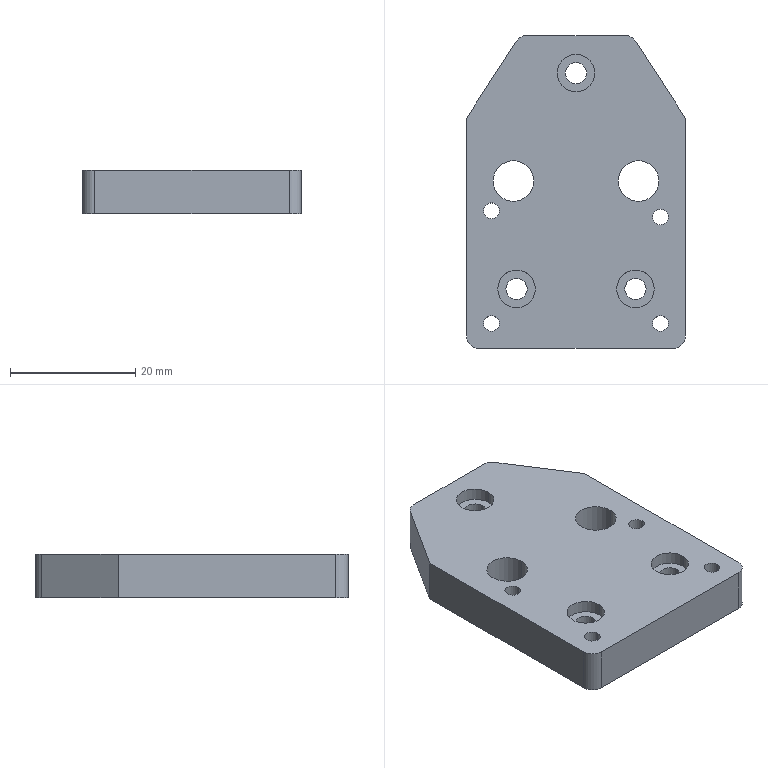Part | STEP file | 11-FG-SB00811 | 1 solid | 48 faces | box 35 x 50 x 7 mm | volume 10258 mm3 | cylinder 34 | plane 14 | commonest cylinder face diameters 2.5 x8 3.4 x6 6 x6 6.5 x6 4 x4 7 x4
STEP:
#1=CARTESIAN_POINT('',(13.25,14.24,7.));
#2=VERTEX_POINT('',#1);
#3=CARTESIAN_POINT('',(6.75,14.24,7.));
#4=VERTEX_POINT('',#3);
#5=CARTESIAN_POINT('',(10.,14.24,7.));
#6=DIRECTION('',(0.,0.,-1.));
#7=DIRECTION('',(-1.,0.,0.));
#8=AXIS2_PLACEMENT_3D('',#5,#6,#7);
#9=CIRCLE('',#8,3.25);
#10=EDGE_CURVE('',#2,#4,#9,.T.);
#11=ORIENTED_EDGE('',*,*,#10,.F.);
#12=CARTESIAN_POINT('',(13.25,14.24,0.));
#13=VERTEX_POINT('',#12);
#14=CARTESIAN_POINT('',(13.25,14.24,7.));
#15=DIRECTION('',(0.,0.,-1.));
#16=VECTOR('',#15,1000.);
#17=LINE('',#14,#16);
#18=EDGE_CURVE('',#2,#13,#17,.T.);
#19=ORIENTED_EDGE('',*,*,#18,.T.);
#20=CARTESIAN_POINT('',(6.75,14.24,0.));
#21=VERTEX_POINT('',#20);
#22=CARTESIAN_POINT('',(10.,14.24,0.));
#23=DIRECTION('',(0.,0.,-1.));
#24=DIRECTION('',(-1.,0.,0.));
#25=AXIS2_PLACEMENT_3D('',#22,#23,#24);
#26=CIRCLE('',#25,3.25);
#27=EDGE_CURVE('',#13,#21,#26,.T.);
#28=ORIENTED_EDGE('',*,*,#27,.T.);
#29=CARTESIAN_POINT('',(6.75,14.24,7.));
#30=DIRECTION('',(0.,0.,-1.));
#31=VECTOR('',#30,1000.);
#32=LINE('',#29,#31);
#33=EDGE_CURVE('',#4,#21,#32,.T.);
#34=ORIENTED_EDGE('',*,*,#33,.F.);
#35=EDGE_LOOP('',(#11,#19,#28,#34));
#36=FACE_OUTER_BOUND('',#35,.T.);
#37=CARTESIAN_POINT('',(10.,14.24,7.));
#38=DIRECTION('',(0.,0.,-1.));
#39=DIRECTION('',(-1.,0.,0.));
#40=AXIS2_PLACEMENT_3D('',#37,#38,#39);
#41=CYLINDRICAL_SURFACE('',#40,3.25);
#42=ADVANCED_FACE('',(#36),#41,.F.);
#43=CARTESIAN_POINT('',(-6.75,14.24,7.));
#44=VERTEX_POINT('',#43);
#45=CARTESIAN_POINT('',(-13.25,14.24,7.));
#46=VERTEX_POINT('',#45);
#47=CARTESIAN_POINT('',(-10.,14.24,7.));
#48=DIRECTION('',(0.,0.,-1.));
#49=DIRECTION('',(-1.,0.,0.));
#50=AXIS2_PLACEMENT_3D('',#47,#48,#49);
#51=CIRCLE('',#50,3.25);
#52=EDGE_CURVE('',#44,#46,#51,.T.);
#53=ORIENTED_EDGE('',*,*,#52,.F.);
#54=CARTESIAN_POINT('',(-6.75,14.24,0.));
#55=VERTEX_POINT('',#54);
#56=CARTESIAN_POINT('',(-6.75,14.24,7.));
#57=DIRECTION('',(0.,0.,-1.));
#58=VECTOR('',#57,1000.);
#59=LINE('',#56,#58);
#60=EDGE_CURVE('',#44,#55,#59,.T.);
#61=ORIENTED_EDGE('',*,*,#60,.T.);
#62=CARTESIAN_POINT('',(-13.25,14.24,0.));
#63=VERTEX_POINT('',#62);
#64=CARTESIAN_POINT('',(-10.,14.24,0.));
#65=DIRECTION('',(0.,0.,-1.));
#66=DIRECTION('',(-1.,0.,0.));
#67=AXIS2_PLACEMENT_3D('',#64,#65,#66);
#68=CIRCLE('',#67,3.25);
#69=EDGE_CURVE('',#55,#63,#68,.T.);
#70=ORIENTED_EDGE('',*,*,#69,.T.);
#71=CARTESIAN_POINT('',(-13.25,14.24,7.));
#72=DIRECTION('',(0.,0.,-1.));
#73=VECTOR('',#72,1000.);
#74=LINE('',#71,#73);
#75=EDGE_CURVE('',#46,#63,#74,.T.);
#76=ORIENTED_EDGE('',*,*,#75,.F.);
#77=EDGE_LOOP('',(#53,#61,#70,#76));
#78=FACE_OUTER_BOUND('',#77,.T.);
#79=CARTESIAN_POINT('',(-10.,14.24,7.));
#80=DIRECTION('',(0.,0.,-1.));
#81=DIRECTION('',(-1.,0.,0.));
#82=AXIS2_PLACEMENT_3D('',#79,#80,#81);
#83=CYLINDRICAL_SURFACE('',#82,3.25);
#84=ADVANCED_FACE('',(#78),#83,.F.);
#85=CARTESIAN_POINT('',(3.25,31.5,3.4));
#86=VERTEX_POINT('',#85);
#87=CARTESIAN_POINT('',(-3.25,31.5,3.4));
#88=VERTEX_POINT('',#87);
#89=CARTESIAN_POINT('',(0.,31.5,3.4));
#90=DIRECTION('',(0.,0.,-1.));
#91=DIRECTION('',(-1.,0.,0.));
#92=AXIS2_PLACEMENT_3D('',#89,#90,#91);
#93=CIRCLE('',#92,3.25);
#94=EDGE_CURVE('',#86,#88,#93,.T.);
#95=ORIENTED_EDGE('',*,*,#94,.F.);
#96=CARTESIAN_POINT('',(3.25,31.5,0.));
#97=VERTEX_POINT('',#96);
#98=CARTESIAN_POINT('',(3.25,31.5,0.));
#99=DIRECTION('',(0.,0.,-1.));
#100=VECTOR('',#99,1000.);
#101=LINE('',#98,#100);
#102=EDGE_CURVE('',#86,#97,#101,.T.);
#103=ORIENTED_EDGE('',*,*,#102,.T.);
#104=CARTESIAN_POINT('',(-3.25,31.5,0.));
#105=VERTEX_POINT('',#104);
#106=CARTESIAN_POINT('',(0.,31.5,0.));
#107=DIRECTION('',(0.,0.,-1.));
#108=DIRECTION('',(-1.,0.,0.));
#109=AXIS2_PLACEMENT_3D('',#106,#107,#108);
#110=CIRCLE('',#109,3.25);
#111=EDGE_CURVE('',#97,#105,#110,.T.);
#112=ORIENTED_EDGE('',*,*,#111,.T.);
#113=CARTESIAN_POINT('',(-3.25,31.5,0.));
#114=DIRECTION('',(0.,0.,-1.));
#115=VECTOR('',#114,1000.);
#116=LINE('',#113,#115);
#117=EDGE_CURVE('',#88,#105,#116,.T.);
#118=ORIENTED_EDGE('',*,*,#117,.F.);
#119=EDGE_LOOP('',(#95,#103,#112,#118));
#120=FACE_OUTER_BOUND('',#119,.T.);
#121=CARTESIAN_POINT('',(0.,31.5,0.));
#122=DIRECTION('',(0.,0.,-1.));
#123=DIRECTION('',(-1.,0.,0.));
#124=AXIS2_PLACEMENT_3D('',#121,#122,#123);
#125=CYLINDRICAL_SURFACE('',#124,3.25);
#126=ADVANCED_FACE('',(#120),#125,.F.);
#127=CARTESIAN_POINT('',(-1.7,31.5,5.));
#128=VERTEX_POINT('',#127);
#129=CARTESIAN_POINT('',(1.7,31.5,5.));
#130=VERTEX_POINT('',#129);
#131=CARTESIAN_POINT('',(0.,31.5,5.));
#132=DIRECTION('',(0.,0.,1.));
#133=DIRECTION('',(1.,0.,0.));
#134=AXIS2_PLACEMENT_3D('',#131,#132,#133);
#135=CIRCLE('',#134,1.7);
#136=EDGE_CURVE('',#128,#130,#135,.T.);
#137=ORIENTED_EDGE('',*,*,#136,.T.);
#138=CARTESIAN_POINT('',(1.7,31.5,3.4));
#139=VERTEX_POINT('',#138);
#140=CARTESIAN_POINT('',(1.7,31.5,0.));
#141=DIRECTION('',(0.,0.,-1.));
#142=VECTOR('',#141,1000.);
#143=LINE('',#140,#142);
#144=EDGE_CURVE('',#130,#139,#143,.T.);
#145=ORIENTED_EDGE('',*,*,#144,.T.);
#146=CARTESIAN_POINT('',(-1.7,31.5,3.4));
#147=VERTEX_POINT('',#146);
#148=CARTESIAN_POINT('',(0.,31.5,3.4));
#149=DIRECTION('',(0.,0.,-1.));
#150=DIRECTION('',(-1.,0.,0.));
#151=AXIS2_PLACEMENT_3D('',#148,#149,#150);
#152=CIRCLE('',#151,1.7);
#153=EDGE_CURVE('',#139,#147,#152,.T.);
#154=ORIENTED_EDGE('',*,*,#153,.T.);
#155=CARTESIAN_POINT('',(-1.7,31.5,0.));
#156=DIRECTION('',(0.,0.,-1.));
#157=VECTOR('',#156,1000.);
#158=LINE('',#155,#157);
#159=EDGE_CURVE('',#128,#147,#158,.T.);
#160=ORIENTED_EDGE('',*,*,#159,.F.);
#161=EDGE_LOOP('',(#137,#145,#154,#160));
#162=FACE_OUTER_BOUND('',#161,.T.);
#163=CARTESIAN_POINT('',(0.,31.5,0.));
#164=DIRECTION('',(0.,0.,-1.));
#165=DIRECTION('',(-1.,0.,0.));
#166=AXIS2_PLACEMENT_3D('',#163,#164,#165);
#167=CYLINDRICAL_SURFACE('',#166,1.7);
#168=ADVANCED_FACE('',(#162),#167,.F.);
#169=CARTESIAN_POINT('',(-3.,31.5,5.));
#170=VERTEX_POINT('',#169);
#171=CARTESIAN_POINT('',(3.,31.5,5.));
#172=VERTEX_POINT('',#171);
#173=CARTESIAN_POINT('',(0.,31.5,5.));
#174=DIRECTION('',(0.,0.,1.));
#175=DIRECTION('',(1.,0.,0.));
#176=AXIS2_PLACEMENT_3D('',#173,#174,#175);
#177=CIRCLE('',#176,3.);
#178=EDGE_CURVE('',#170,#172,#177,.T.);
#179=ORIENTED_EDGE('',*,*,#178,.F.);
#180=CARTESIAN_POINT('',(-3.,31.5,7.));
#181=VERTEX_POINT('',#180);
#182=CARTESIAN_POINT('',(-3.,31.5,5.));
#183=DIRECTION('',(0.,0.,1.));
#184=VECTOR('',#183,1000.);
#185=LINE('',#182,#184);
#186=EDGE_CURVE('',#170,#181,#185,.T.);
#187=ORIENTED_EDGE('',*,*,#186,.T.);
#188=CARTESIAN_POINT('',(3.,31.5,7.));
#189=VERTEX_POINT('',#188);
#190=CARTESIAN_POINT('',(0.,31.5,7.));
#191=DIRECTION('',(0.,0.,1.));
#192=DIRECTION('',(1.,0.,0.));
#193=AXIS2_PLACEMENT_3D('',#190,#191,#192);
#194=CIRCLE('',#193,3.);
#195=EDGE_CURVE('',#181,#189,#194,.T.);
#196=ORIENTED_EDGE('',*,*,#195,.T.);
#197=CARTESIAN_POINT('',(3.,31.5,5.));
#198=DIRECTION('',(0.,0.,1.));
#199=VECTOR('',#198,1000.);
#200=LINE('',#197,#199);
#201=EDGE_CURVE('',#172,#189,#200,.T.);
#202=ORIENTED_EDGE('',*,*,#201,.F.);
#203=EDGE_LOOP('',(#179,#187,#196,#202));
#204=FACE_OUTER_BOUND('',#203,.T.);
#205=CARTESIAN_POINT('',(0.,31.5,5.));
#206=DIRECTION('',(0.,0.,1.));
#207=DIRECTION('',(1.,0.,0.));
#208=AXIS2_PLACEMENT_3D('',#205,#206,#207);
#209=CYLINDRICAL_SURFACE('',#208,3.);
#210=ADVANCED_FACE('',(#204),#209,.F.);
#211=CARTESIAN_POINT('',(-12.25,-8.5,7.));
#212=VERTEX_POINT('',#211);
#213=CARTESIAN_POINT('',(-14.75,-8.5,7.));
#214=VERTEX_POINT('',#213);
#215=CARTESIAN_POINT('',(-13.5,-8.5,7.));
#216=DIRECTION('',(0.,0.,-1.));
#217=DIRECTION('',(-1.,0.,0.));
#218=AXIS2_PLACEMENT_3D('',#215,#216,#217);
#219=CIRCLE('',#218,1.25);
#220=EDGE_CURVE('',#212,#214,#219,.T.);
#221=ORIENTED_EDGE('',*,*,#220,.F.);
#222=CARTESIAN_POINT('',(-12.25,-8.5,0.));
#223=VERTEX_POINT('',#222);
#224=CARTESIAN_POINT('',(-12.25,-8.5,0.));
#225=DIRECTION('',(0.,0.,-1.));
#226=VECTOR('',#225,1000.);
#227=LINE('',#224,#226);
#228=EDGE_CURVE('',#212,#223,#227,.T.);
#229=ORIENTED_EDGE('',*,*,#228,.T.);
#230=CARTESIAN_POINT('',(-14.75,-8.5,0.));
#231=VERTEX_POINT('',#230);
#232=CARTESIAN_POINT('',(-13.5,-8.5,0.));
#233=DIRECTION('',(0.,0.,-1.));
#234=DIRECTION('',(-1.,0.,0.));
#235=AXIS2_PLACEMENT_3D('',#232,#233,#234);
#236=CIRCLE('',#235,1.25);
#237=EDGE_CURVE('',#223,#231,#236,.T.);
#238=ORIENTED_EDGE('',*,*,#237,.T.);
#239=CARTESIAN_POINT('',(-14.75,-8.5,0.));
#240=DIRECTION('',(0.,0.,-1.));
#241=VECTOR('',#240,1000.);
#242=LINE('',#239,#241);
#243=EDGE_CURVE('',#214,#231,#242,.T.);
#244=ORIENTED_EDGE('',*,*,#243,.F.);
#245=EDGE_LOOP('',(#221,#229,#238,#244));
#246=FACE_OUTER_BOUND('',#245,.T.);
#247=CARTESIAN_POINT('',(-13.5,-8.5,0.));
#248=DIRECTION('',(0.,0.,-1.));
#249=DIRECTION('',(-1.,0.,0.));
#250=AXIS2_PLACEMENT_3D('',#247,#248,#249);
#251=CYLINDRICAL_SURFACE('',#250,1.25);
#252=ADVANCED_FACE('',(#246),#251,.F.);
#253=CARTESIAN_POINT('',(14.75,-8.5,7.));
#254=VERTEX_POINT('',#253);
#255=CARTESIAN_POINT('',(12.25,-8.5,7.));
#256=VERTEX_POINT('',#255);
#257=CARTESIAN_POINT('',(13.5,-8.5,7.));
#258=DIRECTION('',(0.,0.,-1.));
#259=DIRECTION('',(-1.,0.,0.));
#260=AXIS2_PLACEMENT_3D('',#257,#258,#259);
#261=CIRCLE('',#260,1.25);
#262=EDGE_CURVE('',#254,#256,#261,.T.);
#263=ORIENTED_EDGE('',*,*,#262,.F.);
#264=CARTESIAN_POINT('',(14.75,-8.5,0.));
#265=VERTEX_POINT('',#264);
#266=CARTESIAN_POINT('',(14.75,-8.5,0.));
#267=DIRECTION('',(0.,0.,-1.));
#268=VECTOR('',#267,1000.);
#269=LINE('',#266,#268);
#270=EDGE_CURVE('',#254,#265,#269,.T.);
#271=ORIENTED_EDGE('',*,*,#270,.T.);
#272=CARTESIAN_POINT('',(12.25,-8.5,0.));
#273=VERTEX_POINT('',#272);
#274=CARTESIAN_POINT('',(13.5,-8.5,0.));
#275=DIRECTION('',(0.,0.,-1.));
#276=DIRECTION('',(-1.,0.,0.));
#277=AXIS2_PLACEMENT_3D('',#274,#275,#276);
#278=CIRCLE('',#277,1.25);
#279=EDGE_CURVE('',#265,#273,#278,.T.);
#280=ORIENTED_EDGE('',*,*,#279,.T.);
#281=CARTESIAN_POINT('',(12.25,-8.5,0.));
#282=DIRECTION('',(0.,0.,-1.));
#283=VECTOR('',#282,1000.);
#284=LINE('',#281,#283);
#285=EDGE_CURVE('',#256,#273,#284,.T.);
#286=ORIENTED_EDGE('',*,*,#285,.F.);
#287=EDGE_LOOP('',(#263,#271,#280,#286));
#288=FACE_OUTER_BOUND('',#287,.T.);
#289=CARTESIAN_POINT('',(13.5,-8.5,0.));
#290=DIRECTION('',(0.,0.,-1.));
#291=DIRECTION('',(-1.,0.,0.));
#292=AXIS2_PLACEMENT_3D('',#289,#290,#291);
#293=CYLINDRICAL_SURFACE('',#292,1.25);
#294=ADVANCED_FACE('',(#288),#293,.F.);
#295=CARTESIAN_POINT('',(14.75,8.5,7.));
#296=VERTEX_POINT('',#295);
#297=CARTESIAN_POINT('',(12.25,8.5,7.));
#298=VERTEX_POINT('',#297);
#299=CARTESIAN_POINT('',(13.5,8.5,7.));
#300=DIRECTION('',(0.,0.,-1.));
#301=DIRECTION('',(-1.,0.,0.));
#302=AXIS2_PLACEMENT_3D('',#299,#300,#301);
#303=CIRCLE('',#302,1.25);
#304=EDGE_CURVE('',#296,#298,#303,.T.);
#305=ORIENTED_EDGE('',*,*,#304,.F.);
#306=CARTESIAN_POINT('',(14.75,8.5,0.));
#307=VERTEX_POINT('',#306);
#308=CARTESIAN_POINT('',(14.75,8.5,0.));
#309=DIRECTION('',(0.,0.,-1.));
#310=VECTOR('',#309,1000.);
#311=LINE('',#308,#310);
#312=EDGE_CURVE('',#296,#307,#311,.T.);
#313=ORIENTED_EDGE('',*,*,#312,.T.);
#314=CARTESIAN_POINT('',(12.25,8.5,0.));
#315=VERTEX_POINT('',#314);
#316=CARTESIAN_POINT('',(13.5,8.5,0.));
#317=DIRECTION('',(0.,0.,-1.));
#318=DIRECTION('',(-1.,0.,0.));
#319=AXIS2_PLACEMENT_3D('',#316,#317,#318);
#320=CIRCLE('',#319,1.25);
#321=EDGE_CURVE('',#307,#315,#320,.T.);
#322=ORIENTED_EDGE('',*,*,#321,.T.);
#323=CARTESIAN_POINT('',(12.25,8.5,0.));
#324=DIRECTION('',(0.,0.,-1.));
#325=VECTOR('',#324,1000.);
#326=LINE('',#323,#325);
#327=EDGE_CURVE('',#298,#315,#326,.T.);
#328=ORIENTED_EDGE('',*,*,#327,.F.);
#329=EDGE_LOOP('',(#305,#313,#322,#328));
#330=FACE_OUTER_BOUND('',#329,.T.);
#331=CARTESIAN_POINT('',(13.5,8.5,0.));
#332=DIRECTION('',(0.,0.,-1.));
#333=DIRECTION('',(-1.,0.,0.));
#334=AXIS2_PLACEMENT_3D('',#331,#332,#333);
#335=CYLINDRICAL_SURFACE('',#334,1.25);
#336=ADVANCED_FACE('',(#330),#335,.F.);
#337=CARTESIAN_POINT('',(-12.25,9.5,7.));
#338=VERTEX_POINT('',#337);
#339=CARTESIAN_POINT('',(-14.75,9.5,7.));
#340=VERTEX_POINT('',#339);
#341=CARTESIAN_POINT('',(-13.5,9.5,7.));
#342=DIRECTION('',(0.,0.,-1.));
#343=DIRECTION('',(-1.,0.,0.));
#344=AXIS2_PLACEMENT_3D('',#341,#342,#343);
#345=CIRCLE('',#344,1.25);
#346=EDGE_CURVE('',#338,#340,#345,.T.);
#347=ORIENTED_EDGE('',*,*,#346,.F.);
#348=CARTESIAN_POINT('',(-12.25,9.5,0.));
#349=VERTEX_POINT('',#348);
#350=CARTESIAN_POINT('',(-12.25,9.5,0.));
#351=DIRECTION('',(0.,0.,-1.));
#352=VECTOR('',#351,1000.);
#353=LINE('',#350,#352);
#354=EDGE_CURVE('',#338,#349,#353,.T.);
#355=ORIENTED_EDGE('',*,*,#354,.T.);
#356=CARTESIAN_POINT('',(-14.75,9.5,0.));
#357=VERTEX_POINT('',#356);
#358=CARTESIAN_POINT('',(-13.5,9.5,0.));
#359=DIRECTION('',(0.,0.,-1.));
#360=DIRECTION('',(-1.,0.,0.));
#361=AXIS2_PLACEMENT_3D('',#358,#359,#360);
#362=CIRCLE('',#361,1.25);
#363=EDGE_CURVE('',#349,#357,#362,.T.);
#364=ORIENTED_EDGE('',*,*,#363,.T.);
#365=CARTESIAN_POINT('',(-14.75,9.5,0.));
#366=DIRECTION('',(0.,0.,-1.));
#367=VECTOR('',#366,1000.);
#368=LINE('',#365,#367);
#369=EDGE_CURVE('',#340,#357,#368,.T.);
#370=ORIENTED_EDGE('',*,*,#369,.F.);
#371=EDGE_LOOP('',(#347,#355,#364,#370));
#372=FACE_OUTER_BOUND('',#371,.T.);
#373=CARTESIAN_POINT('',(-13.5,9.5,0.));
#374=DIRECTION('',(0.,0.,-1.));
#375=DIRECTION('',(-1.,0.,0.));
#376=AXIS2_PLACEMENT_3D('',#373,#374,#375);
#377=CYLINDRICAL_SURFACE('',#376,1.25);
#378=ADVANCED_FACE('',(#372),#377,.F.);
#379=CARTESIAN_POINT('',(-6.,-3.,3.4));
#380=VERTEX_POINT('',#379);
#381=CARTESIAN_POINT('',(-13.,-3.,3.4));
#382=VERTEX_POINT('',#381);
#383=CARTESIAN_POINT('',(-9.5,-3.,3.4));
#384=DIRECTION('',(0.,0.,-1.));
#385=DIRECTION('',(-1.,0.,0.));
#386=AXIS2_PLACEMENT_3D('',#383,#384,#385);
#387=CIRCLE('',#386,3.5);
#388=EDGE_CURVE('',#380,#382,#387,.T.);
#389=ORIENTED_EDGE('',*,*,#388,.F.);
#390=CARTESIAN_POINT('',(-6.,-3.,0.));
#391=VERTEX_POINT('',#390);
#392=CARTESIAN_POINT('',(-6.,-3.,0.));
#393=DIRECTION('',(0.,0.,-1.));
#394=VECTOR('',#393,1000.);
#395=LINE('',#392,#394);
#396=EDGE_CURVE('',#380,#391,#395,.T.);
#397=ORIENTED_EDGE('',*,*,#396,.T.);
#398=CARTESIAN_POINT('',(-13.,-3.,0.));
#399=VERTEX_POINT('',#398);
#400=CARTESIAN_POINT('',(-9.5,-3.,0.));
#401=DIRECTION('',(0.,0.,-1.));
#402=DIRECTION('',(-1.,0.,0.));
#403=AXIS2_PLACEMENT_3D('',#400,#401,#402);
#404=CIRCLE('',#403,3.5);
#405=EDGE_CURVE('',#391,#399,#404,.T.);
#406=ORIENTED_EDGE('',*,*,#405,.T.);
#407=CARTESIAN_POINT('',(-13.,-3.,0.));
#408=DIRECTION('',(0.,0.,-1.));
#409=VECTOR('',#408,1000.);
#410=LINE('',#407,#409);
#411=EDGE_CURVE('',#382,#399,#410,.T.);
#412=ORIENTED_EDGE('',*,*,#411,.F.);
#413=EDGE_LOOP('',(#389,#397,#406,#412));
#414=FACE_OUTER_BOUND('',#413,.T.);
#415=CARTESIAN_POINT('',(-9.5,-3.,0.));
#416=DIRECTION('',(0.,0.,-1.));
#417=DIRECTION('',(-1.,0.,0.));
#418=AXIS2_PLACEMENT_3D('',#415,#416,#417);
#419=CYLINDRICAL_SURFACE('',#418,3.5);
#420=ADVANCED_FACE('',(#414),#419,.F.);
#421=CARTESIAN_POINT('',(-7.8,-3.,5.));
#422=VERTEX_POINT('',#421);
#423=CARTESIAN_POINT('',(-11.2,-3.,5.));
#424=VERTEX_POINT('',#423);
#425=CARTESIAN_POINT('',(-9.5,-3.,5.));
#426=DIRECTION('',(0.,0.,-1.));
#427=DIRECTION('',(-1.,0.,0.));
#428=AXIS2_PLACEMENT_3D('',#425,#426,#427);
#429=CIRCLE('',#428,1.7);
#430=EDGE_CURVE('',#422,#424,#429,.T.);
#431=ORIENTED_EDGE('',*,*,#430,.F.);
#432=CARTESIAN_POINT('',(-7.8,-3.,3.4));
#433=VERTEX_POINT('',#432);
#434=CARTESIAN_POINT('',(-7.8,-3.,0.));
#435=DIRECTION('',(0.,0.,-1.));
#436=VECTOR('',#435,1000.);
#437=LINE('',#434,#436);
#438=EDGE_CURVE('',#422,#433,#437,.T.);
#439=ORIENTED_EDGE('',*,*,#438,.T.);
#440=CARTESIAN_POINT('',(-11.2,-3.,3.4));
#441=VERTEX_POINT('',#440);
#442=CARTESIAN_POINT('',(-9.5,-3.,3.4));
#443=DIRECTION('',(0.,0.,-1.));
#444=DIRECTION('',(-1.,0.,0.));
#445=AXIS2_PLACEMENT_3D('',#442,#443,#444);
#446=CIRCLE('',#445,1.7);
#447=EDGE_CURVE('',#433,#441,#446,.T.);
#448=ORIENTED_EDGE('',*,*,#447,.T.);
#449=CARTESIAN_POINT('',(-11.2,-3.,0.));
#450=DIRECTION('',(0.,0.,-1.));
#451=VECTOR('',#450,1000.);
#452=LINE('',#449,#451);
#453=EDGE_CURVE('',#424,#441,#452,.T.);
#454=ORIENTED_EDGE('',*,*,#453,.F.);
#455=EDGE_LOOP('',(#431,#439,#448,#454));
#456=FACE_OUTER_BOUND('',#455,.T.);
#457=CARTESIAN_POINT('',(-9.5,-3.,0.));
#458=DIRECTION('',(0.,0.,-1.));
#459=DIRECTION('',(-1.,0.,0.));
#460=AXIS2_PLACEMENT_3D('',#457,#458,#459);
#461=CYLINDRICAL_SURFACE('',#460,1.7);
#462=ADVANCED_FACE('',(#456),#461,.F.);
#463=CARTESIAN_POINT('',(13.,-3.,3.4));
#464=VERTEX_POINT('',#463);
#465=CARTESIAN_POINT('',(6.,-3.,3.4));
#466=VERTEX_POINT('',#465);
#467=CARTESIAN_POINT('',(9.5,-3.,3.4));
#468=DIRECTION('',(0.,0.,-1.));
#469=DIRECTION('',(-1.,0.,0.));
#470=AXIS2_PLACEMENT_3D('',#467,#468,#469);
#471=CIRCLE('',#470,3.5);
#472=EDGE_CURVE('',#464,#466,#471,.T.);
#473=ORIENTED_EDGE('',*,*,#472,.F.);
#474=CARTESIAN_POINT('',(13.,-3.,0.));
#475=VERTEX_POINT('',#474);
#476=CARTESIAN_POINT('',(13.,-3.,0.));
#477=DIRECTION('',(0.,0.,-1.));
#478=VECTOR('',#477,1000.);
#479=LINE('',#476,#478);
#480=EDGE_CURVE('',#464,#475,#479,.T.);
#481=ORIENTED_EDGE('',*,*,#480,.T.);
#482=CARTESIAN_POINT('',(6.,-3.,0.));
#483=VERTEX_POINT('',#482);
#484=CARTESIAN_POINT('',(9.5,-3.,0.));
#485=DIRECTION('',(0.,0.,-1.));
#486=DIRECTION('',(-1.,0.,0.));
#487=AXIS2_PLACEMENT_3D('',#484,#485,#486);
#488=CIRCLE('',#487,3.5);
#489=EDGE_CURVE('',#475,#483,#488,.T.);
#490=ORIENTED_EDGE('',*,*,#489,.T.);
#491=CARTESIAN_POINT('',(6.,-3.,0.));
#492=DIRECTION('',(0.,0.,-1.));
#493=VECTOR('',#492,1000.);
#494=LINE('',#491,#493);
#495=EDGE_CURVE('',#466,#483,#494,.T.);
#496=ORIENTED_EDGE('',*,*,#495,.F.);
#497=EDGE_LOOP('',(#473,#481,#490,#496));
#498=FACE_OUTER_BOUND('',#497,.T.);
#499=CARTESIAN_POINT('',(9.5,-3.,0.));
#500=DIRECTION('',(0.,0.,-1.));
#501=DIRECTION('',(-1.,0.,0.));
#502=AXIS2_PLACEMENT_3D('',#499,#500,#501);
#503=CYLINDRICAL_SURFACE('',#502,3.5);
#504=ADVANCED_FACE('',(#498),#503,.F.);
#505=CARTESIAN_POINT('',(7.8,-3.,5.));
#506=VERTEX_POINT('',#505);
#507=CARTESIAN_POINT('',(11.2,-3.,5.));
#508=VERTEX_POINT('',#507);
#509=CARTESIAN_POINT('',(9.5,-3.,5.));
#510=DIRECTION('',(0.,0.,1.));
#511=DIRECTION('',(1.,0.,0.));
#512=AXIS2_PLACEMENT_3D('',#509,#510,#511);
#513=CIRCLE('',#512,1.7);
#514=EDGE_CURVE('',#506,#508,#513,.T.);
#515=ORIENTED_EDGE('',*,*,#514,.T.);
#516=CARTESIAN_POINT('',(11.2,-3.,3.4));
#517=VERTEX_POINT('',#516);
#518=CARTESIAN_POINT('',(11.2,-3.,0.));
#519=DIRECTION('',(0.,0.,-1.));
#520=VECTOR('',#519,1000.);
#521=LINE('',#518,#520);
#522=EDGE_CURVE('',#508,#517,#521,.T.);
#523=ORIENTED_EDGE('',*,*,#522,.T.);
#524=CARTESIAN_POINT('',(7.8,-3.,3.4));
#525=VERTEX_POINT('',#524);
#526=CARTESIAN_POINT('',(9.5,-3.,3.4));
#527=DIRECTION('',(0.,0.,-1.));
#528=DIRECTION('',(-1.,0.,0.));
#529=AXIS2_PLACEMENT_3D('',#526,#527,#528);
#530=CIRCLE('',#529,1.7);
#531=EDGE_CURVE('',#517,#525,#530,.T.);
#532=ORIENTED_EDGE('',*,*,#531,.T.);
#533=CARTESIAN_POINT('',(7.8,-3.,0.));
#534=DIRECTION('',(0.,0.,-1.));
#535=VECTOR('',#534,1000.);
#536=LINE('',#533,#535);
#537=EDGE_CURVE('',#506,#525,#536,.T.);
#538=ORIENTED_EDGE('',*,*,#537,.F.);
#539=EDGE_LOOP('',(#515,#523,#532,#538));
#540=FACE_OUTER_BOUND('',#539,.T.);
#541=CARTESIAN_POINT('',(9.5,-3.,0.));
#542=DIRECTION('',(0.,0.,-1.));
#543=DIRECTION('',(-1.,0.,0.));
#544=AXIS2_PLACEMENT_3D('',#541,#542,#543);
#545=CYLINDRICAL_SURFACE('',#544,1.7);
#546=ADVANCED_FACE('',(#540),#545,.F.);
#547=CARTESIAN_POINT('',(-12.5,-3.,5.));
#548=VERTEX_POINT('',#547);
#549=CARTESIAN_POINT('',(-6.5,-3.,5.));
#550=VERTEX_POINT('',#549);
#551=CARTESIAN_POINT('',(-9.5,-3.,5.));
#552=DIRECTION('',(0.,0.,1.));
#553=DIRECTION('',(-1.,0.,0.));
#554=AXIS2_PLACEMENT_3D('',#551,#552,#553);
#555=CIRCLE('',#554,3.);
#556=EDGE_CURVE('',#548,#550,#555,.T.);
#557=ORIENTED_EDGE('',*,*,#556,.F.);
#558=CARTESIAN_POINT('',(-12.5,-3.,7.));
#559=VERTEX_POINT('',#558);
#560=CARTESIAN_POINT('',(-12.5,-3.,5.));
#561=DIRECTION('',(0.,0.,1.));
#562=VECTOR('',#561,1000.);
#563=LINE('',#560,#562);
#564=EDGE_CURVE('',#548,#559,#563,.T.);
#565=ORIENTED_EDGE('',*,*,#564,.T.);
#566=CARTESIAN_POINT('',(-6.5,-3.,7.));
#567=VERTEX_POINT('',#566);
#568=CARTESIAN_POINT('',(-9.5,-3.,7.));
#569=DIRECTION('',(0.,0.,1.));
#570=DIRECTION('',(-1.,0.,0.));
#571=AXIS2_PLACEMENT_3D('',#568,#569,#570);
#572=CIRCLE('',#571,3.);
#573=EDGE_CURVE('',#559,#567,#572,.T.);
#574=ORIENTED_EDGE('',*,*,#573,.T.);
#575=CARTESIAN_POINT('',(-6.5,-3.,5.));
#576=DIRECTION('',(0.,0.,1.));
#577=VECTOR('',#576,1000.);
#578=LINE('',#575,#577);
#579=EDGE_CURVE('',#550,#567,#578,.T.);
#580=ORIENTED_EDGE('',*,*,#579,.F.);
#581=EDGE_LOOP('',(#557,#565,#574,#580));
#582=FACE_OUTER_BOUND('',#581,.T.);
#583=CARTESIAN_POINT('',(-9.5,-3.,5.));
#584=DIRECTION('',(0.,0.,1.));
#585=DIRECTION('',(1.,0.,0.));
#586=AXIS2_PLACEMENT_3D('',#583,#584,#585);
#587=CYLINDRICAL_SURFACE('',#586,3.);
#588=ADVANCED_FACE('',(#582),#587,.F.);
#589=CARTESIAN_POINT('',(6.5,-3.,5.));
#590=VERTEX_POINT('',#589);
#591=CARTESIAN_POINT('',(12.5,-3.,5.));
#592=VERTEX_POINT('',#591);
#593=CARTESIAN_POINT('',(9.5,-3.,5.));
#594=DIRECTION('',(0.,0.,1.));
#595=DIRECTION('',(1.,0.,0.));
#596=AXIS2_PLACEMENT_3D('',#593,#594,#595);
#597=CIRCLE('',#596,3.);
#598=EDGE_CURVE('',#590,#592,#597,.T.);
#599=ORIENTED_EDGE('',*,*,#598,.F.);
#600=CARTESIAN_POINT('',(6.5,-3.,7.));
#601=VERTEX_POINT('',#600);
#602=CARTESIAN_POINT('',(6.5,-3.,5.));
#603=DIRECTION('',(0.,0.,1.));
#604=VECTOR('',#603,1000.);
#605=LINE('',#602,#604);
#606=EDGE_CURVE('',#590,#601,#605,.T.);
#607=ORIENTED_EDGE('',*,*,#606,.T.);
#608=CARTESIAN_POINT('',(12.5,-3.,7.));
#609=VERTEX_POINT('',#608);
#610=CARTESIAN_POINT('',(9.5,-3.,7.));
#611=DIRECTION('',(0.,0.,1.));
#612=DIRECTION('',(1.,0.,0.));
#613=AXIS2_PLACEMENT_3D('',#610,#611,#612);
#614=CIRCLE('',#613,3.);
#615=EDGE_CURVE('',#601,#609,#614,.T.);
#616=ORIENTED_EDGE('',*,*,#615,.T.);
#617=CARTESIAN_POINT('',(12.5,-3.,5.));
#618=DIRECTION('',(0.,0.,1.));
#619=VECTOR('',#618,1000.);
#620=LINE('',#617,#619);
#621=EDGE_CURVE('',#592,#609,#620,.T.);
#622=ORIENTED_EDGE('',*,*,#621,.F.);
#623=EDGE_LOOP('',(#599,#607,#616,#622));
#624=FACE_OUTER_BOUND('',#623,.T.);
#625=CARTESIAN_POINT('',(9.5,-3.,5.));
#626=DIRECTION('',(0.,0.,1.));
#627=DIRECTION('',(1.,0.,0.));
#628=AXIS2_PLACEMENT_3D('',#625,#626,#627);
#629=CYLINDRICAL_SURFACE('',#628,3.);
#630=ADVANCED_FACE('',(#624),#629,.F.);
#631=CARTESIAN_POINT('',(17.5,-10.5,7.));
#632=VERTEX_POINT('',#631);
#633=CARTESIAN_POINT('',(17.5,24.29,7.));
#634=VERTEX_POINT('',#633);
#635=CARTESIAN_POINT('',(17.5,12.5,7.));
#636=DIRECTION('',(0.,1.,0.));
#637=VECTOR('',#636,1000.);
#638=LINE('',#635,#637);
#639=EDGE_CURVE('',#632,#634,#638,.T.);
#640=ORIENTED_EDGE('',*,*,#639,.F.);
#641=CARTESIAN_POINT('',(17.5,-10.5,0.));
#642=VERTEX_POINT('',#641);
#643=CARTESIAN_POINT('',(17.5,-10.5,7.));
#644=DIRECTION('',(0.,0.,-1.));
#645=VECTOR('',#644,1000.);
#646=LINE('',#643,#645);
#647=EDGE_CURVE('',#632,#642,#646,.T.);
#648=ORIENTED_EDGE('',*,*,#647,.T.);
#649=CARTESIAN_POINT('',(17.5,24.29,0.));
#650=VERTEX_POINT('',#649);
#651=CARTESIAN_POINT('',(17.5,12.5,0.));
#652=DIRECTION('',(0.,1.,0.));
#653=VECTOR('',#652,1000.);
#654=LINE('',#651,#653);
#655=EDGE_CURVE('',#642,#650,#654,.T.);
#656=ORIENTED_EDGE('',*,*,#655,.T.);
#657=CARTESIAN_POINT('',(17.5,24.29,0.));
#658=DIRECTION('',(0.,0.,1.));
#659=VECTOR('',#658,1000.);
#660=LINE('',#657,#659);
#661=EDGE_CURVE('',#650,#634,#660,.T.);
#662=ORIENTED_EDGE('',*,*,#661,.T.);
#663=EDGE_LOOP('',(#640,#648,#656,#662));
#664=FACE_OUTER_BOUND('',#663,.T.);
#665=CARTESIAN_POINT('',(17.5,12.5,7.));
#666=DIRECTION('',(-1.,0.,0.));
#667=DIRECTION('',(0.,-1.,0.));
#668=AXIS2_PLACEMENT_3D('',#665,#666,#667);
#669=PLANE('',#668);
#670=ADVANCED_FACE('',(#664),#669,.F.);
#671=CARTESIAN_POINT('',(-17.5,24.29,0.));
#672=VERTEX_POINT('',#671);
#673=CARTESIAN_POINT('',(-17.5,-10.5,0.));
#674=VERTEX_POINT('',#673);
#675=CARTESIAN_POINT('',(-17.5,12.5,0.));
#676=DIRECTION('',(0.,-1.,0.));
#677=VECTOR('',#676,1000.);
#678=LINE('',#675,#677);
#679=EDGE_CURVE('',#672,#674,#678,.T.);
#680=ORIENTED_EDGE('',*,*,#679,.T.);
#681=CARTESIAN_POINT('',(-17.5,-10.5,7.));
#682=VERTEX_POINT('',#681);
#683=CARTESIAN_POINT('',(-17.5,-10.5,7.));
#684=DIRECTION('',(0.,0.,1.));
#685=VECTOR('',#684,1000.);
#686=LINE('',#683,#685);
#687=EDGE_CURVE('',#674,#682,#686,.T.);
#688=ORIENTED_EDGE('',*,*,#687,.T.);
#689=CARTESIAN_POINT('',(-17.5,24.29,7.));
#690=VERTEX_POINT('',#689);
#691=CARTESIAN_POINT('',(-17.5,12.5,7.));
#692=DIRECTION('',(0.,-1.,0.));
#693=VECTOR('',#692,1000.);
#694=LINE('',#691,#693);
#695=EDGE_CURVE('',#690,#682,#694,.T.);
#696=ORIENTED_EDGE('',*,*,#695,.F.);
#697=CARTESIAN_POINT('',(-17.5,24.29,0.));
#698=DIRECTION('',(0.,0.,1.));
#699=VECTOR('',#698,1000.);
#700=LINE('',#697,#699);
#701=EDGE_CURVE('',#672,#690,#700,.T.);
#702=ORIENTED_EDGE('',*,*,#701,.F.);
#703=EDGE_LOOP('',(#680,#688,#696,#702));
#704=FACE_OUTER_BOUND('',#703,.T.);
#705=CARTESIAN_POINT('',(-17.5,12.5,7.));
#706=DIRECTION('',(1.,0.,0.));
#707=DIRECTION('',(0.,1.,0.));
#708=AXIS2_PLACEMENT_3D('',#705,#706,#707);
#709=PLANE('',#708);
#710=ADVANCED_FACE('',(#704),#709,.F.);
#711=CARTESIAN_POINT('',(-15.5,-12.5,0.));
#712=VERTEX_POINT('',#711);
#713=CARTESIAN_POINT('',(15.5,-12.5,0.));
#714=VERTEX_POINT('',#713);
#715=CARTESIAN_POINT('',(-17.5,-12.5,0.));
#716=DIRECTION('',(1.,0.,0.));
#717=VECTOR('',#716,1000.);
#718=LINE('',#715,#717);
#719=EDGE_CURVE('',#712,#714,#718,.T.);
#720=ORIENTED_EDGE('',*,*,#719,.T.);
#721=CARTESIAN_POINT('',(15.5,-12.5,7.));
#722=VERTEX_POINT('',#721);
#723=CARTESIAN_POINT('',(15.5,-12.5,7.));
#724=DIRECTION('',(0.,0.,1.));
#725=VECTOR('',#724,1000.);
#726=LINE('',#723,#725);
#727=EDGE_CURVE('',#714,#722,#726,.T.);
#728=ORIENTED_EDGE('',*,*,#727,.T.);
#729=CARTESIAN_POINT('',(-15.5,-12.5,7.));
#730=VERTEX_POINT('',#729);
#731=CARTESIAN_POINT('',(-17.5,-12.5,7.));
#732=DIRECTION('',(1.,0.,0.));
#733=VECTOR('',#732,1000.);
#734=LINE('',#731,#733);
#735=EDGE_CURVE('',#730,#722,#734,.T.);
#736=ORIENTED_EDGE('',*,*,#735,.F.);
#737=CARTESIAN_POINT('',(-15.5,-12.5,7.));
#738=DIRECTION('',(0.,0.,-1.));
#739=VECTOR('',#738,1000.);
#740=LINE('',#737,#739);
#741=EDGE_CURVE('',#730,#712,#740,.T.);
#742=ORIENTED_EDGE('',*,*,#741,.T.);
#743=EDGE_LOOP('',(#720,#728,#736,#742));
#744=FACE_OUTER_BOUND('',#743,.T.);
#745=CARTESIAN_POINT('',(-17.5,-12.5,7.));
#746=DIRECTION('',(0.,1.,0.));
#747=DIRECTION('',(0.,0.,1.));
#748=AXIS2_PLACEMENT_3D('',#745,#746,#747);
#749=PLANE('',#748);
#750=ADVANCED_FACE('',(#744),#749,.F.);
#751=CARTESIAN_POINT('',(10.,14.24,7.));
#752=DIRECTION('',(0.,0.,-1.));
#753=DIRECTION('',(-1.,0.,0.));
#754=AXIS2_PLACEMENT_3D('',#751,#752,#753);
#755=CIRCLE('',#754,3.25);
#756=EDGE_CURVE('',#4,#2,#755,.T.);
#757=ORIENTED_EDGE('',*,*,#756,.T.);
#758=ORIENTED_EDGE('',*,*,#10,.T.);
#759=EDGE_LOOP('',(#757,#758));
#760=FACE_BOUND('',#759,.T.);
#761=CARTESIAN_POINT('',(-10.,14.24,7.));
#762=DIRECTION('',(0.,0.,-1.));
#763=DIRECTION('',(-1.,0.,0.));
#764=AXIS2_PLACEMENT_3D('',#761,#762,#763);
#765=CIRCLE('',#764,3.25);
#766=EDGE_CURVE('',#46,#44,#765,.T.);
#767=ORIENTED_EDGE('',*,*,#766,.T.);
#768=ORIENTED_EDGE('',*,*,#52,.T.);
#769=EDGE_LOOP('',(#767,#768));
#770=FACE_BOUND('',#769,.T.);
#771=CARTESIAN_POINT('',(9.568,36.584,7.));
#772=VERTEX_POINT('',#771);
#773=CARTESIAN_POINT('',(17.5,24.29,7.));
#774=DIRECTION('',(0.5421,-0.8403,0.));
#775=VECTOR('',#774,1000.);
#776=LINE('',#773,#775);
#777=EDGE_CURVE('',#772,#634,#776,.T.);
#778=ORIENTED_EDGE('',*,*,#777,.F.);
#779=CARTESIAN_POINT('',(7.888,37.5,7.));
#780=VERTEX_POINT('',#779);
#781=CARTESIAN_POINT('',(7.888,35.5,7.));
#782=DIRECTION('',(0.,0.,1.));
#783=DIRECTION('',(1.,0.,0.));
#784=AXIS2_PLACEMENT_3D('',#781,#782,#783);
#785=CIRCLE('',#784,2.);
#786=EDGE_CURVE('',#772,#780,#785,.T.);
#787=ORIENTED_EDGE('',*,*,#786,.T.);
#788=CARTESIAN_POINT('',(-7.888,37.5,7.));
#789=VERTEX_POINT('',#788);
#790=CARTESIAN_POINT('',(17.5,37.5,7.));
#791=DIRECTION('',(1.,0.,0.));
#792=VECTOR('',#791,1000.);
#793=LINE('',#790,#792);
#794=EDGE_CURVE('',#789,#780,#793,.T.);
#795=ORIENTED_EDGE('',*,*,#794,.F.);
#796=CARTESIAN_POINT('',(-9.568,36.584,7.));
#797=VERTEX_POINT('',#796);
#798=CARTESIAN_POINT('',(-7.888,35.5,7.));
#799=DIRECTION('',(0.,0.,1.));
#800=DIRECTION('',(1.,0.,0.));
#801=AXIS2_PLACEMENT_3D('',#798,#799,#800);
#802=CIRCLE('',#801,2.);
#803=EDGE_CURVE('',#789,#797,#802,.T.);
#804=ORIENTED_EDGE('',*,*,#803,.T.);
#805=CARTESIAN_POINT('',(-17.5,24.29,7.));
#806=DIRECTION('',(0.5421,0.8403,0.));
#807=VECTOR('',#806,1000.);
#808=LINE('',#805,#807);
#809=EDGE_CURVE('',#690,#797,#808,.T.);
#810=ORIENTED_EDGE('',*,*,#809,.F.);
#811=ORIENTED_EDGE('',*,*,#695,.T.);
#812=CARTESIAN_POINT('',(-15.5,-10.5,7.));
#813=DIRECTION('',(0.,0.,1.));
#814=DIRECTION('',(1.,0.,0.));
#815=AXIS2_PLACEMENT_3D('',#812,#813,#814);
#816=CIRCLE('',#815,2.);
#817=EDGE_CURVE('',#682,#730,#816,.T.);
#818=ORIENTED_EDGE('',*,*,#817,.T.);
#819=ORIENTED_EDGE('',*,*,#735,.T.);
#820=CARTESIAN_POINT('',(15.5,-10.5,7.));
#821=DIRECTION('',(0.,0.,1.));
#822=DIRECTION('',(1.,0.,0.));
#823=AXIS2_PLACEMENT_3D('',#820,#821,#822);
#824=CIRCLE('',#823,2.);
#825=EDGE_CURVE('',#722,#632,#824,.T.);
#826=ORIENTED_EDGE('',*,*,#825,.T.);
#827=ORIENTED_EDGE('',*,*,#639,.T.);
#828=EDGE_LOOP('',(#778,#787,#795,#804,#810,#811,#818,#819,#826,#827));
#829=FACE_OUTER_BOUND('',#828,.T.);
#830=CARTESIAN_POINT('',(0.,31.5,7.));
#831=DIRECTION('',(0.,0.,1.));
#832=DIRECTION('',(1.,0.,0.));
#833=AXIS2_PLACEMENT_3D('',#830,#831,#832);
#834=CIRCLE('',#833,3.);
#835=EDGE_CURVE('',#189,#181,#834,.T.);
#836=ORIENTED_EDGE('',*,*,#835,.F.);
#837=ORIENTED_EDGE('',*,*,#195,.F.);
#838=EDGE_LOOP('',(#836,#837));
#839=FACE_BOUND('',#838,.T.);
#840=CARTESIAN_POINT('',(-13.5,-8.5,7.));
#841=DIRECTION('',(0.,0.,-1.));
#842=DIRECTION('',(-1.,0.,0.));
#843=AXIS2_PLACEMENT_3D('',#840,#841,#842);
#844=CIRCLE('',#843,1.25);
#845=EDGE_CURVE('',#214,#212,#844,.T.);
#846=ORIENTED_EDGE('',*,*,#845,.T.);
#847=ORIENTED_EDGE('',*,*,#220,.T.);
#848=EDGE_LOOP('',(#846,#847));
#849=FACE_BOUND('',#848,.T.);
#850=CARTESIAN_POINT('',(13.5,-8.5,7.));
#851=DIRECTION('',(0.,0.,-1.));
#852=DIRECTION('',(-1.,0.,0.));
#853=AXIS2_PLACEMENT_3D('',#850,#851,#852);
#854=CIRCLE('',#853,1.25);
#855=EDGE_CURVE('',#256,#254,#854,.T.);
#856=ORIENTED_EDGE('',*,*,#855,.T.);
#857=ORIENTED_EDGE('',*,*,#262,.T.);
#858=EDGE_LOOP('',(#856,#857));
#859=FACE_BOUND('',#858,.T.);
#860=CARTESIAN_POINT('',(13.5,8.5,7.));
#861=DIRECTION('',(0.,0.,-1.));
#862=DIRECTION('',(-1.,0.,0.));
#863=AXIS2_PLACEMENT_3D('',#860,#861,#862);
#864=CIRCLE('',#863,1.25);
#865=EDGE_CURVE('',#298,#296,#864,.T.);
#866=ORIENTED_EDGE('',*,*,#865,.T.);
#867=ORIENTED_EDGE('',*,*,#304,.T.);
#868=EDGE_LOOP('',(#866,#867));
#869=FACE_BOUND('',#868,.T.);
#870=CARTESIAN_POINT('',(-13.5,9.5,7.));
#871=DIRECTION('',(0.,0.,-1.));
#872=DIRECTION('',(-1.,0.,0.));
#873=AXIS2_PLACEMENT_3D('',#870,#871,#872);
#874=CIRCLE('',#873,1.25);
#875=EDGE_CURVE('',#340,#338,#874,.T.);
#876=ORIENTED_EDGE('',*,*,#875,.T.);
#877=ORIENTED_EDGE('',*,*,#346,.T.);
#878=EDGE_LOOP('',(#876,#877));
#879=FACE_BOUND('',#878,.T.);
#880=CARTESIAN_POINT('',(-9.5,-3.,7.));
#881=DIRECTION('',(0.,0.,1.));
#882=DIRECTION('',(-1.,0.,0.));
#883=AXIS2_PLACEMENT_3D('',#880,#881,#882);
#884=CIRCLE('',#883,3.);
#885=EDGE_CURVE('',#567,#559,#884,.T.);
#886=ORIENTED_EDGE('',*,*,#885,.F.);
#887=ORIENTED_EDGE('',*,*,#573,.F.);
#888=EDGE_LOOP('',(#886,#887));
#889=FACE_BOUND('',#888,.T.);
#890=CARTESIAN_POINT('',(9.5,-3.,7.));
#891=DIRECTION('',(0.,0.,1.));
#892=DIRECTION('',(1.,0.,0.));
#893=AXIS2_PLACEMENT_3D('',#890,#891,#892);
#894=CIRCLE('',#893,3.);
#895=EDGE_CURVE('',#609,#601,#894,.T.);
#896=ORIENTED_EDGE('',*,*,#895,.F.);
#897=ORIENTED_EDGE('',*,*,#615,.F.);
#898=EDGE_LOOP('',(#896,#897));
#899=FACE_BOUND('',#898,.T.);
#900=CARTESIAN_POINT('',(0.,0.,7.));
#901=DIRECTION('',(0.,0.,1.));
#902=DIRECTION('',(1.,0.,0.));
#903=AXIS2_PLACEMENT_3D('',#900,#901,#902);
#904=PLANE('',#903);
#905=ADVANCED_FACE('',(#760,#770,#829,#839,#849,#859,#869,#879,#889,#899),#904,.T.);
#906=CARTESIAN_POINT('',(10.,14.24,0.));
#907=DIRECTION('',(0.,0.,-1.));
#908=DIRECTION('',(-1.,0.,0.));
#909=AXIS2_PLACEMENT_3D('',#906,#907,#908);
#910=CIRCLE('',#909,3.25);
#911=EDGE_CURVE('',#21,#13,#910,.T.);
#912=ORIENTED_EDGE('',*,*,#911,.F.);
#913=ORIENTED_EDGE('',*,*,#27,.F.);
#914=EDGE_LOOP('',(#912,#913));
#915=FACE_BOUND('',#914,.T.);
#916=CARTESIAN_POINT('',(-10.,14.24,0.));
#917=DIRECTION('',(0.,0.,-1.));
#918=DIRECTION('',(-1.,0.,0.));
#919=AXIS2_PLACEMENT_3D('',#916,#917,#918);
#920=CIRCLE('',#919,3.25);
#921=EDGE_CURVE('',#63,#55,#920,.T.);
#922=ORIENTED_EDGE('',*,*,#921,.F.);
#923=ORIENTED_EDGE('',*,*,#69,.F.);
#924=EDGE_LOOP('',(#922,#923));
#925=FACE_BOUND('',#924,.T.);
#926=CARTESIAN_POINT('',(0.,31.5,0.));
#927=DIRECTION('',(0.,0.,-1.));
#928=DIRECTION('',(-1.,0.,0.));
#929=AXIS2_PLACEMENT_3D('',#926,#927,#928);
#930=CIRCLE('',#929,3.25);
#931=EDGE_CURVE('',#105,#97,#930,.T.);
#932=ORIENTED_EDGE('',*,*,#931,.F.);
#933=ORIENTED_EDGE('',*,*,#111,.F.);
#934=EDGE_LOOP('',(#932,#933));
#935=FACE_BOUND('',#934,.T.);
#936=CARTESIAN_POINT('',(-13.5,-8.5,0.));
#937=DIRECTION('',(0.,0.,-1.));
#938=DIRECTION('',(-1.,0.,0.));
#939=AXIS2_PLACEMENT_3D('',#936,#937,#938);
#940=CIRCLE('',#939,1.25);
#941=EDGE_CURVE('',#231,#223,#940,.T.);
#942=ORIENTED_EDGE('',*,*,#941,.F.);
#943=ORIENTED_EDGE('',*,*,#237,.F.);
#944=EDGE_LOOP('',(#942,#943));
#945=FACE_BOUND('',#944,.T.);
#946=CARTESIAN_POINT('',(13.5,-8.5,0.));
#947=DIRECTION('',(0.,0.,-1.));
#948=DIRECTION('',(-1.,0.,0.));
#949=AXIS2_PLACEMENT_3D('',#946,#947,#948);
#950=CIRCLE('',#949,1.25);
#951=EDGE_CURVE('',#273,#265,#950,.T.);
#952=ORIENTED_EDGE('',*,*,#951,.F.);
#953=ORIENTED_EDGE('',*,*,#279,.F.);
#954=EDGE_LOOP('',(#952,#953));
#955=FACE_BOUND('',#954,.T.);
#956=CARTESIAN_POINT('',(13.5,8.5,0.));
#957=DIRECTION('',(0.,0.,-1.));
#958=DIRECTION('',(-1.,0.,0.));
#959=AXIS2_PLACEMENT_3D('',#956,#957,#958);
#960=CIRCLE('',#959,1.25);
#961=EDGE_CURVE('',#315,#307,#960,.T.);
#962=ORIENTED_EDGE('',*,*,#961,.F.);
#963=ORIENTED_EDGE('',*,*,#321,.F.);
#964=EDGE_LOOP('',(#962,#963));
#965=FACE_BOUND('',#964,.T.);
#966=CARTESIAN_POINT('',(-13.5,9.5,0.));
#967=DIRECTION('',(0.,0.,-1.));
#968=DIRECTION('',(-1.,0.,0.));
#969=AXIS2_PLACEMENT_3D('',#966,#967,#968);
#970=CIRCLE('',#969,1.25);
#971=EDGE_CURVE('',#357,#349,#970,.T.);
#972=ORIENTED_EDGE('',*,*,#971,.F.);
#973=ORIENTED_EDGE('',*,*,#363,.F.);
#974=EDGE_LOOP('',(#972,#973));
#975=FACE_BOUND('',#974,.T.);
#976=CARTESIAN_POINT('',(-9.5,-3.,0.));
#977=DIRECTION('',(0.,0.,-1.));
#978=DIRECTION('',(-1.,0.,0.));
#979=AXIS2_PLACEMENT_3D('',#976,#977,#978);
#980=CIRCLE('',#979,3.5);
#981=EDGE_CURVE('',#399,#391,#980,.T.);
#982=ORIENTED_EDGE('',*,*,#981,.F.);
#983=ORIENTED_EDGE('',*,*,#405,.F.);
#984=EDGE_LOOP('',(#982,#983));
#985=FACE_BOUND('',#984,.T.);
#986=CARTESIAN_POINT('',(9.5,-3.,0.));
#987=DIRECTION('',(0.,0.,-1.));
#988=DIRECTION('',(-1.,0.,0.));
#989=AXIS2_PLACEMENT_3D('',#986,#987,#988);
#990=CIRCLE('',#989,3.5);
#991=EDGE_CURVE('',#483,#475,#990,.T.);
#992=ORIENTED_EDGE('',*,*,#991,.F.);
#993=ORIENTED_EDGE('',*,*,#489,.F.);
#994=EDGE_LOOP('',(#992,#993));
#995=FACE_BOUND('',#994,.T.);
#996=CARTESIAN_POINT('',(7.888,37.5,0.));
#997=VERTEX_POINT('',#996);
#998=CARTESIAN_POINT('',(-7.888,37.5,0.));
#999=VERTEX_POINT('',#998);
#1000=CARTESIAN_POINT('',(17.5,37.5,0.));
#1001=DIRECTION('',(-1.,0.,0.));
#1002=VECTOR('',#1001,1000.);
#1003=LINE('',#1000,#1002);
#1004=EDGE_CURVE('',#997,#999,#1003,.T.);
#1005=ORIENTED_EDGE('',*,*,#1004,.F.);
#1006=CARTESIAN_POINT('',(9.568,36.584,0.));
#1007=VERTEX_POINT('',#1006);
#1008=CARTESIAN_POINT('',(7.888,35.5,0.));
#1009=DIRECTION('',(0.,0.,-1.));
#1010=DIRECTION('',(1.,0.,0.));
#1011=AXIS2_PLACEMENT_3D('',#1008,#1009,#1010);
#1012=CIRCLE('',#1011,2.);
#1013=EDGE_CURVE('',#997,#1007,#1012,.T.);
#1014=ORIENTED_EDGE('',*,*,#1013,.T.);
#1015=CARTESIAN_POINT('',(17.5,24.29,0.));
#1016=DIRECTION('',(0.5421,-0.8403,0.));
#1017=VECTOR('',#1016,1000.);
#1018=LINE('',#1015,#1017);
#1019=EDGE_CURVE('',#1007,#650,#1018,.T.);
#1020=ORIENTED_EDGE('',*,*,#1019,.T.);
#1021=ORIENTED_EDGE('',*,*,#655,.F.);
#1022=CARTESIAN_POINT('',(15.5,-10.5,0.));
#1023=DIRECTION('',(0.,0.,-1.));
#1024=DIRECTION('',(1.,0.,0.));
#1025=AXIS2_PLACEMENT_3D('',#1022,#1023,#1024);
#1026=CIRCLE('',#1025,2.);
#1027=EDGE_CURVE('',#642,#714,#1026,.T.);
#1028=ORIENTED_EDGE('',*,*,#1027,.T.);
#1029=ORIENTED_EDGE('',*,*,#719,.F.);
#1030=CARTESIAN_POINT('',(-15.5,-10.5,0.));
#1031=DIRECTION('',(0.,0.,-1.));
#1032=DIRECTION('',(1.,0.,0.));
#1033=AXIS2_PLACEMENT_3D('',#1030,#1031,#1032);
#1034=CIRCLE('',#1033,2.);
#1035=EDGE_CURVE('',#712,#674,#1034,.T.);
#1036=ORIENTED_EDGE('',*,*,#1035,.T.);
#1037=ORIENTED_EDGE('',*,*,#679,.F.);
#1038=CARTESIAN_POINT('',(-9.568,36.584,0.));
#1039=VERTEX_POINT('',#1038);
#1040=CARTESIAN_POINT('',(-17.5,24.29,0.));
#1041=DIRECTION('',(0.5421,0.8403,0.));
#1042=VECTOR('',#1041,1000.);
#1043=LINE('',#1040,#1042);
#1044=EDGE_CURVE('',#672,#1039,#1043,.T.);
#1045=ORIENTED_EDGE('',*,*,#1044,.T.);
#1046=CARTESIAN_POINT('',(-7.888,35.5,0.));
#1047=DIRECTION('',(0.,0.,-1.));
#1048=DIRECTION('',(1.,0.,0.));
#1049=AXIS2_PLACEMENT_3D('',#1046,#1047,#1048);
#1050=CIRCLE('',#1049,2.);
#1051=EDGE_CURVE('',#1039,#999,#1050,.T.);
#1052=ORIENTED_EDGE('',*,*,#1051,.T.);
#1053=EDGE_LOOP('',(#1005,#1014,#1020,#1021,#1028,#1029,#1036,#1037,#1045,#1052));
#1054=FACE_OUTER_BOUND('',#1053,.T.);
#1055=CARTESIAN_POINT('',(0.,0.,0.));
#1056=DIRECTION('',(0.,0.,1.));
#1057=DIRECTION('',(1.,0.,0.));
#1058=AXIS2_PLACEMENT_3D('',#1055,#1056,#1057);
#1059=PLANE('',#1058);
#1060=ADVANCED_FACE('',(#915,#925,#935,#945,#955,#965,#975,#985,#995,#1054),#1059,.F.);
#1061=ORIENTED_EDGE('',*,*,#606,.F.);
#1062=CARTESIAN_POINT('',(9.5,-3.,5.));
#1063=DIRECTION('',(0.,0.,1.));
#1064=DIRECTION('',(1.,0.,0.));
#1065=AXIS2_PLACEMENT_3D('',#1062,#1063,#1064);
#1066=CIRCLE('',#1065,3.);
#1067=EDGE_CURVE('',#592,#590,#1066,.T.);
#1068=ORIENTED_EDGE('',*,*,#1067,.F.);
#1069=ORIENTED_EDGE('',*,*,#621,.T.);
#1070=ORIENTED_EDGE('',*,*,#895,.T.);
#1071=EDGE_LOOP('',(#1061,#1068,#1069,#1070));
#1072=FACE_OUTER_BOUND('',#1071,.T.);
#1073=CARTESIAN_POINT('',(9.5,-3.,5.));
#1074=DIRECTION('',(0.,0.,1.));
#1075=DIRECTION('',(1.,0.,0.));
#1076=AXIS2_PLACEMENT_3D('',#1073,#1074,#1075);
#1077=CYLINDRICAL_SURFACE('',#1076,3.);
#1078=ADVANCED_FACE('',(#1072),#1077,.F.);
#1079=ORIENTED_EDGE('',*,*,#514,.F.);
#1080=CARTESIAN_POINT('',(9.5,-3.,5.));
#1081=DIRECTION('',(0.,0.,1.));
#1082=DIRECTION('',(1.,0.,0.));
#1083=AXIS2_PLACEMENT_3D('',#1080,#1081,#1082);
#1084=CIRCLE('',#1083,1.7);
#1085=EDGE_CURVE('',#508,#506,#1084,.T.);
#1086=ORIENTED_EDGE('',*,*,#1085,.F.);
#1087=EDGE_LOOP('',(#1079,#1086));
#1088=FACE_BOUND('',#1087,.T.);
#1089=ORIENTED_EDGE('',*,*,#1067,.T.);
#1090=ORIENTED_EDGE('',*,*,#598,.T.);
#1091=EDGE_LOOP('',(#1089,#1090));
#1092=FACE_OUTER_BOUND('',#1091,.T.);
#1093=CARTESIAN_POINT('',(9.5,-3.,5.));
#1094=DIRECTION('',(0.,0.,1.));
#1095=DIRECTION('',(1.,0.,0.));
#1096=AXIS2_PLACEMENT_3D('',#1093,#1094,#1095);
#1097=PLANE('',#1096);
#1098=ADVANCED_FACE('',(#1088,#1092),#1097,.T.);
#1099=ORIENTED_EDGE('',*,*,#564,.F.);
#1100=CARTESIAN_POINT('',(-9.5,-3.,5.));
#1101=DIRECTION('',(0.,0.,1.));
#1102=DIRECTION('',(-1.,0.,0.));
#1103=AXIS2_PLACEMENT_3D('',#1100,#1101,#1102);
#1104=CIRCLE('',#1103,3.);
#1105=EDGE_CURVE('',#550,#548,#1104,.T.);
#1106=ORIENTED_EDGE('',*,*,#1105,.F.);
#1107=ORIENTED_EDGE('',*,*,#579,.T.);
#1108=ORIENTED_EDGE('',*,*,#885,.T.);
#1109=EDGE_LOOP('',(#1099,#1106,#1107,#1108));
#1110=FACE_OUTER_BOUND('',#1109,.T.);
#1111=CARTESIAN_POINT('',(-9.5,-3.,5.));
#1112=DIRECTION('',(0.,0.,1.));
#1113=DIRECTION('',(1.,0.,0.));
#1114=AXIS2_PLACEMENT_3D('',#1111,#1112,#1113);
#1115=CYLINDRICAL_SURFACE('',#1114,3.);
#1116=ADVANCED_FACE('',(#1110),#1115,.F.);
#1117=CARTESIAN_POINT('',(-9.5,-3.,5.));
#1118=DIRECTION('',(0.,0.,-1.));
#1119=DIRECTION('',(-1.,0.,0.));
#1120=AXIS2_PLACEMENT_3D('',#1117,#1118,#1119);
#1121=CIRCLE('',#1120,1.7);
#1122=EDGE_CURVE('',#424,#422,#1121,.T.);
#1123=ORIENTED_EDGE('',*,*,#1122,.T.);
#1124=ORIENTED_EDGE('',*,*,#430,.T.);
#1125=EDGE_LOOP('',(#1123,#1124));
#1126=FACE_BOUND('',#1125,.T.);
#1127=ORIENTED_EDGE('',*,*,#1105,.T.);
#1128=ORIENTED_EDGE('',*,*,#556,.T.);
#1129=EDGE_LOOP('',(#1127,#1128));
#1130=FACE_OUTER_BOUND('',#1129,.T.);
#1131=CARTESIAN_POINT('',(-9.5,-3.,5.));
#1132=DIRECTION('',(0.,0.,-1.));
#1133=DIRECTION('',(-1.,0.,0.));
#1134=AXIS2_PLACEMENT_3D('',#1131,#1132,#1133);
#1135=PLANE('',#1134);
#1136=ADVANCED_FACE('',(#1126,#1130),#1135,.F.);
#1137=ORIENTED_EDGE('',*,*,#522,.F.);
#1138=ORIENTED_EDGE('',*,*,#1085,.T.);
#1139=ORIENTED_EDGE('',*,*,#537,.T.);
#1140=CARTESIAN_POINT('',(9.5,-3.,3.4));
#1141=DIRECTION('',(0.,0.,-1.));
#1142=DIRECTION('',(-1.,0.,0.));
#1143=AXIS2_PLACEMENT_3D('',#1140,#1141,#1142);
#1144=CIRCLE('',#1143,1.7);
#1145=EDGE_CURVE('',#525,#517,#1144,.T.);
#1146=ORIENTED_EDGE('',*,*,#1145,.T.);
#1147=EDGE_LOOP('',(#1137,#1138,#1139,#1146));
#1148=FACE_OUTER_BOUND('',#1147,.T.);
#1149=CARTESIAN_POINT('',(9.5,-3.,0.));
#1150=DIRECTION('',(0.,0.,-1.));
#1151=DIRECTION('',(-1.,0.,0.));
#1152=AXIS2_PLACEMENT_3D('',#1149,#1150,#1151);
#1153=CYLINDRICAL_SURFACE('',#1152,1.7);
#1154=ADVANCED_FACE('',(#1148),#1153,.F.);
#1155=ORIENTED_EDGE('',*,*,#1145,.F.);
#1156=ORIENTED_EDGE('',*,*,#531,.F.);
#1157=EDGE_LOOP('',(#1155,#1156));
#1158=FACE_BOUND('',#1157,.T.);
#1159=CARTESIAN_POINT('',(9.5,-3.,3.4));
#1160=DIRECTION('',(0.,0.,-1.));
#1161=DIRECTION('',(-1.,0.,0.));
#1162=AXIS2_PLACEMENT_3D('',#1159,#1160,#1161);
#1163=CIRCLE('',#1162,3.5);
#1164=EDGE_CURVE('',#466,#464,#1163,.T.);
#1165=ORIENTED_EDGE('',*,*,#1164,.T.);
#1166=ORIENTED_EDGE('',*,*,#472,.T.);
#1167=EDGE_LOOP('',(#1165,#1166));
#1168=FACE_OUTER_BOUND('',#1167,.T.);
#1169=CARTESIAN_POINT('',(11.2,-3.,3.4));
#1170=DIRECTION('',(0.,0.,1.));
#1171=DIRECTION('',(1.,0.,0.));
#1172=AXIS2_PLACEMENT_3D('',#1169,#1170,#1171);
#1173=PLANE('',#1172);
#1174=ADVANCED_FACE('',(#1158,#1168),#1173,.F.);
#1175=ORIENTED_EDGE('',*,*,#480,.F.);
#1176=ORIENTED_EDGE('',*,*,#1164,.F.);
#1177=ORIENTED_EDGE('',*,*,#495,.T.);
#1178=ORIENTED_EDGE('',*,*,#991,.T.);
#1179=EDGE_LOOP('',(#1175,#1176,#1177,#1178));
#1180=FACE_OUTER_BOUND('',#1179,.T.);
#1181=CARTESIAN_POINT('',(9.5,-3.,0.));
#1182=DIRECTION('',(0.,0.,-1.));
#1183=DIRECTION('',(-1.,0.,0.));
#1184=AXIS2_PLACEMENT_3D('',#1181,#1182,#1183);
#1185=CYLINDRICAL_SURFACE('',#1184,3.5);
#1186=ADVANCED_FACE('',(#1180),#1185,.F.);
#1187=ORIENTED_EDGE('',*,*,#438,.F.);
#1188=ORIENTED_EDGE('',*,*,#1122,.F.);
#1189=ORIENTED_EDGE('',*,*,#453,.T.);
#1190=CARTESIAN_POINT('',(-9.5,-3.,3.4));
#1191=DIRECTION('',(0.,0.,-1.));
#1192=DIRECTION('',(-1.,0.,0.));
#1193=AXIS2_PLACEMENT_3D('',#1190,#1191,#1192);
#1194=CIRCLE('',#1193,1.7);
#1195=EDGE_CURVE('',#441,#433,#1194,.T.);
#1196=ORIENTED_EDGE('',*,*,#1195,.T.);
#1197=EDGE_LOOP('',(#1187,#1188,#1189,#1196));
#1198=FACE_OUTER_BOUND('',#1197,.T.);
#1199=CARTESIAN_POINT('',(-9.5,-3.,0.));
#1200=DIRECTION('',(0.,0.,-1.));
#1201=DIRECTION('',(-1.,0.,0.));
#1202=AXIS2_PLACEMENT_3D('',#1199,#1200,#1201);
#1203=CYLINDRICAL_SURFACE('',#1202,1.7);
#1204=ADVANCED_FACE('',(#1198),#1203,.F.);
#1205=ORIENTED_EDGE('',*,*,#1195,.F.);
#1206=ORIENTED_EDGE('',*,*,#447,.F.);
#1207=EDGE_LOOP('',(#1205,#1206));
#1208=FACE_BOUND('',#1207,.T.);
#1209=CARTESIAN_POINT('',(-9.5,-3.,3.4));
#1210=DIRECTION('',(0.,0.,-1.));
#1211=DIRECTION('',(-1.,0.,0.));
#1212=AXIS2_PLACEMENT_3D('',#1209,#1210,#1211);
#1213=CIRCLE('',#1212,3.5);
#1214=EDGE_CURVE('',#382,#380,#1213,.T.);
#1215=ORIENTED_EDGE('',*,*,#1214,.T.);
#1216=ORIENTED_EDGE('',*,*,#388,.T.);
#1217=EDGE_LOOP('',(#1215,#1216));
#1218=FACE_OUTER_BOUND('',#1217,.T.);
#1219=CARTESIAN_POINT('',(-7.8,-3.,3.4));
#1220=DIRECTION('',(0.,0.,1.));
#1221=DIRECTION('',(1.,0.,0.));
#1222=AXIS2_PLACEMENT_3D('',#1219,#1220,#1221);
#1223=PLANE('',#1222);
#1224=ADVANCED_FACE('',(#1208,#1218),#1223,.F.);
#1225=ORIENTED_EDGE('',*,*,#396,.F.);
#1226=ORIENTED_EDGE('',*,*,#1214,.F.);
#1227=ORIENTED_EDGE('',*,*,#411,.T.);
#1228=ORIENTED_EDGE('',*,*,#981,.T.);
#1229=EDGE_LOOP('',(#1225,#1226,#1227,#1228));
#1230=FACE_OUTER_BOUND('',#1229,.T.);
#1231=CARTESIAN_POINT('',(-9.5,-3.,0.));
#1232=DIRECTION('',(0.,0.,-1.));
#1233=DIRECTION('',(-1.,0.,0.));
#1234=AXIS2_PLACEMENT_3D('',#1231,#1232,#1233);
#1235=CYLINDRICAL_SURFACE('',#1234,3.5);
#1236=ADVANCED_FACE('',(#1230),#1235,.F.);
#1237=ORIENTED_EDGE('',*,*,#354,.F.);
#1238=ORIENTED_EDGE('',*,*,#875,.F.);
#1239=ORIENTED_EDGE('',*,*,#369,.T.);
#1240=ORIENTED_EDGE('',*,*,#971,.T.);
#1241=EDGE_LOOP('',(#1237,#1238,#1239,#1240));
#1242=FACE_OUTER_BOUND('',#1241,.T.);
#1243=CARTESIAN_POINT('',(-13.5,9.5,0.));
#1244=DIRECTION('',(0.,0.,-1.));
#1245=DIRECTION('',(-1.,0.,0.));
#1246=AXIS2_PLACEMENT_3D('',#1243,#1244,#1245);
#1247=CYLINDRICAL_SURFACE('',#1246,1.25);
#1248=ADVANCED_FACE('',(#1242),#1247,.F.);
#1249=ORIENTED_EDGE('',*,*,#312,.F.);
#1250=ORIENTED_EDGE('',*,*,#865,.F.);
#1251=ORIENTED_EDGE('',*,*,#327,.T.);
#1252=ORIENTED_EDGE('',*,*,#961,.T.);
#1253=EDGE_LOOP('',(#1249,#1250,#1251,#1252));
#1254=FACE_OUTER_BOUND('',#1253,.T.);
#1255=CARTESIAN_POINT('',(13.5,8.5,0.));
#1256=DIRECTION('',(0.,0.,-1.));
#1257=DIRECTION('',(-1.,0.,0.));
#1258=AXIS2_PLACEMENT_3D('',#1255,#1256,#1257);
#1259=CYLINDRICAL_SURFACE('',#1258,1.25);
#1260=ADVANCED_FACE('',(#1254),#1259,.F.);
#1261=ORIENTED_EDGE('',*,*,#270,.F.);
#1262=ORIENTED_EDGE('',*,*,#855,.F.);
#1263=ORIENTED_EDGE('',*,*,#285,.T.);
#1264=ORIENTED_EDGE('',*,*,#951,.T.);
#1265=EDGE_LOOP('',(#1261,#1262,#1263,#1264));
#1266=FACE_OUTER_BOUND('',#1265,.T.);
#1267=CARTESIAN_POINT('',(13.5,-8.5,0.));
#1268=DIRECTION('',(0.,0.,-1.));
#1269=DIRECTION('',(-1.,0.,0.));
#1270=AXIS2_PLACEMENT_3D('',#1267,#1268,#1269);
#1271=CYLINDRICAL_SURFACE('',#1270,1.25);
#1272=ADVANCED_FACE('',(#1266),#1271,.F.);
#1273=ORIENTED_EDGE('',*,*,#228,.F.);
#1274=ORIENTED_EDGE('',*,*,#845,.F.);
#1275=ORIENTED_EDGE('',*,*,#243,.T.);
#1276=ORIENTED_EDGE('',*,*,#941,.T.);
#1277=EDGE_LOOP('',(#1273,#1274,#1275,#1276));
#1278=FACE_OUTER_BOUND('',#1277,.T.);
#1279=CARTESIAN_POINT('',(-13.5,-8.5,0.));
#1280=DIRECTION('',(0.,0.,-1.));
#1281=DIRECTION('',(-1.,0.,0.));
#1282=AXIS2_PLACEMENT_3D('',#1279,#1280,#1281);
#1283=CYLINDRICAL_SURFACE('',#1282,1.25);
#1284=ADVANCED_FACE('',(#1278),#1283,.F.);
#1285=ORIENTED_EDGE('',*,*,#794,.T.);
#1286=CARTESIAN_POINT('',(7.888,37.5,0.));
#1287=DIRECTION('',(0.,0.,-1.));
#1288=VECTOR('',#1287,1000.);
#1289=LINE('',#1286,#1288);
#1290=EDGE_CURVE('',#780,#997,#1289,.T.);
#1291=ORIENTED_EDGE('',*,*,#1290,.T.);
#1292=ORIENTED_EDGE('',*,*,#1004,.T.);
#1293=CARTESIAN_POINT('',(-7.888,37.5,7.));
#1294=DIRECTION('',(0.,0.,1.));
#1295=VECTOR('',#1294,1000.);
#1296=LINE('',#1293,#1295);
#1297=EDGE_CURVE('',#999,#789,#1296,.T.);
#1298=ORIENTED_EDGE('',*,*,#1297,.T.);
#1299=EDGE_LOOP('',(#1285,#1291,#1292,#1298));
#1300=FACE_OUTER_BOUND('',#1299,.T.);
#1301=CARTESIAN_POINT('',(0.,37.5,0.));
#1302=DIRECTION('',(0.,1.,0.));
#1303=DIRECTION('',(0.,0.,1.));
#1304=AXIS2_PLACEMENT_3D('',#1301,#1302,#1303);
#1305=PLANE('',#1304);
#1306=ADVANCED_FACE('',(#1300),#1305,.T.);
#1307=ORIENTED_EDGE('',*,*,#186,.F.);
#1308=CARTESIAN_POINT('',(0.,31.5,5.));
#1309=DIRECTION('',(0.,0.,1.));
#1310=DIRECTION('',(1.,0.,0.));
#1311=AXIS2_PLACEMENT_3D('',#1308,#1309,#1310);
#1312=CIRCLE('',#1311,3.);
#1313=EDGE_CURVE('',#172,#170,#1312,.T.);
#1314=ORIENTED_EDGE('',*,*,#1313,.F.);
#1315=ORIENTED_EDGE('',*,*,#201,.T.);
#1316=ORIENTED_EDGE('',*,*,#835,.T.);
#1317=EDGE_LOOP('',(#1307,#1314,#1315,#1316));
#1318=FACE_OUTER_BOUND('',#1317,.T.);
#1319=CARTESIAN_POINT('',(0.,31.5,5.));
#1320=DIRECTION('',(0.,0.,1.));
#1321=DIRECTION('',(1.,0.,0.));
#1322=AXIS2_PLACEMENT_3D('',#1319,#1320,#1321);
#1323=CYLINDRICAL_SURFACE('',#1322,3.);
#1324=ADVANCED_FACE('',(#1318),#1323,.F.);
#1325=ORIENTED_EDGE('',*,*,#136,.F.);
#1326=CARTESIAN_POINT('',(0.,31.5,5.));
#1327=DIRECTION('',(0.,0.,1.));
#1328=DIRECTION('',(1.,0.,0.));
#1329=AXIS2_PLACEMENT_3D('',#1326,#1327,#1328);
#1330=CIRCLE('',#1329,1.7);
#1331=EDGE_CURVE('',#130,#128,#1330,.T.);
#1332=ORIENTED_EDGE('',*,*,#1331,.F.);
#1333=EDGE_LOOP('',(#1325,#1332));
#1334=FACE_BOUND('',#1333,.T.);
#1335=ORIENTED_EDGE('',*,*,#1313,.T.);
#1336=ORIENTED_EDGE('',*,*,#178,.T.);
#1337=EDGE_LOOP('',(#1335,#1336));
#1338=FACE_OUTER_BOUND('',#1337,.T.);
#1339=CARTESIAN_POINT('',(0.,31.5,5.));
#1340=DIRECTION('',(0.,0.,1.));
#1341=DIRECTION('',(1.,0.,0.));
#1342=AXIS2_PLACEMENT_3D('',#1339,#1340,#1341);
#1343=PLANE('',#1342);
#1344=ADVANCED_FACE('',(#1334,#1338),#1343,.T.);
#1345=ORIENTED_EDGE('',*,*,#144,.F.);
#1346=ORIENTED_EDGE('',*,*,#1331,.T.);
#1347=ORIENTED_EDGE('',*,*,#159,.T.);
#1348=CARTESIAN_POINT('',(0.,31.5,3.4));
#1349=DIRECTION('',(0.,0.,-1.));
#1350=DIRECTION('',(-1.,0.,0.));
#1351=AXIS2_PLACEMENT_3D('',#1348,#1349,#1350);
#1352=CIRCLE('',#1351,1.7);
#1353=EDGE_CURVE('',#147,#139,#1352,.T.);
#1354=ORIENTED_EDGE('',*,*,#1353,.T.);
#1355=EDGE_LOOP('',(#1345,#1346,#1347,#1354));
#1356=FACE_OUTER_BOUND('',#1355,.T.);
#1357=CARTESIAN_POINT('',(0.,31.5,0.));
#1358=DIRECTION('',(0.,0.,-1.));
#1359=DIRECTION('',(-1.,0.,0.));
#1360=AXIS2_PLACEMENT_3D('',#1357,#1358,#1359);
#1361=CYLINDRICAL_SURFACE('',#1360,1.7);
#1362=ADVANCED_FACE('',(#1356),#1361,.F.);
#1363=ORIENTED_EDGE('',*,*,#1353,.F.);
#1364=ORIENTED_EDGE('',*,*,#153,.F.);
#1365=EDGE_LOOP('',(#1363,#1364));
#1366=FACE_BOUND('',#1365,.T.);
#1367=CARTESIAN_POINT('',(0.,31.5,3.4));
#1368=DIRECTION('',(0.,0.,-1.));
#1369=DIRECTION('',(-1.,0.,0.));
#1370=AXIS2_PLACEMENT_3D('',#1367,#1368,#1369);
#1371=CIRCLE('',#1370,3.25);
#1372=EDGE_CURVE('',#88,#86,#1371,.T.);
#1373=ORIENTED_EDGE('',*,*,#1372,.T.);
#1374=ORIENTED_EDGE('',*,*,#94,.T.);
#1375=EDGE_LOOP('',(#1373,#1374));
#1376=FACE_OUTER_BOUND('',#1375,.T.);
#1377=CARTESIAN_POINT('',(1.7,31.5,3.4));
#1378=DIRECTION('',(0.,0.,1.));
#1379=DIRECTION('',(1.,0.,0.));
#1380=AXIS2_PLACEMENT_3D('',#1377,#1378,#1379);
#1381=PLANE('',#1380);
#1382=ADVANCED_FACE('',(#1366,#1376),#1381,.F.);
#1383=ORIENTED_EDGE('',*,*,#102,.F.);
#1384=ORIENTED_EDGE('',*,*,#1372,.F.);
#1385=ORIENTED_EDGE('',*,*,#117,.T.);
#1386=ORIENTED_EDGE('',*,*,#931,.T.);
#1387=EDGE_LOOP('',(#1383,#1384,#1385,#1386));
#1388=FACE_OUTER_BOUND('',#1387,.T.);
#1389=CARTESIAN_POINT('',(0.,31.5,0.));
#1390=DIRECTION('',(0.,0.,-1.));
#1391=DIRECTION('',(-1.,0.,0.));
#1392=AXIS2_PLACEMENT_3D('',#1389,#1390,#1391);
#1393=CYLINDRICAL_SURFACE('',#1392,3.25);
#1394=ADVANCED_FACE('',(#1388),#1393,.F.);
#1395=ORIENTED_EDGE('',*,*,#1019,.F.);
#1396=CARTESIAN_POINT('',(9.568,36.584,7.));
#1397=DIRECTION('',(0.,0.,1.));
#1398=VECTOR('',#1397,1000.);
#1399=LINE('',#1396,#1398);
#1400=EDGE_CURVE('',#1007,#772,#1399,.T.);
#1401=ORIENTED_EDGE('',*,*,#1400,.T.);
#1402=ORIENTED_EDGE('',*,*,#777,.T.);
#1403=ORIENTED_EDGE('',*,*,#661,.F.);
#1404=EDGE_LOOP('',(#1395,#1401,#1402,#1403));
#1405=FACE_OUTER_BOUND('',#1404,.T.);
#1406=CARTESIAN_POINT('',(17.5,24.29,0.));
#1407=DIRECTION('',(-0.8403,-0.5421,0.));
#1408=DIRECTION('',(0.5421,-0.8403,0.));
#1409=AXIS2_PLACEMENT_3D('',#1406,#1407,#1408);
#1410=PLANE('',#1409);
#1411=ADVANCED_FACE('',(#1405),#1410,.F.);
#1412=ORIENTED_EDGE('',*,*,#809,.T.);
#1413=CARTESIAN_POINT('',(-9.568,36.584,0.));
#1414=DIRECTION('',(0.,0.,-1.));
#1415=VECTOR('',#1414,1000.);
#1416=LINE('',#1413,#1415);
#1417=EDGE_CURVE('',#797,#1039,#1416,.T.);
#1418=ORIENTED_EDGE('',*,*,#1417,.T.);
#1419=ORIENTED_EDGE('',*,*,#1044,.F.);
#1420=ORIENTED_EDGE('',*,*,#701,.T.);
#1421=EDGE_LOOP('',(#1412,#1418,#1419,#1420));
#1422=FACE_OUTER_BOUND('',#1421,.T.);
#1423=CARTESIAN_POINT('',(-17.5,24.29,0.));
#1424=DIRECTION('',(0.8403,-0.5421,0.));
#1425=DIRECTION('',(0.5421,0.8403,0.));
#1426=AXIS2_PLACEMENT_3D('',#1423,#1424,#1425);
#1427=PLANE('',#1426);
#1428=ADVANCED_FACE('',(#1422),#1427,.F.);
#1429=ORIENTED_EDGE('',*,*,#60,.F.);
#1430=ORIENTED_EDGE('',*,*,#766,.F.);
#1431=ORIENTED_EDGE('',*,*,#75,.T.);
#1432=ORIENTED_EDGE('',*,*,#921,.T.);
#1433=EDGE_LOOP('',(#1429,#1430,#1431,#1432));
#1434=FACE_OUTER_BOUND('',#1433,.T.);
#1435=CARTESIAN_POINT('',(-10.,14.24,7.));
#1436=DIRECTION('',(0.,0.,-1.));
#1437=DIRECTION('',(-1.,0.,0.));
#1438=AXIS2_PLACEMENT_3D('',#1435,#1436,#1437);
#1439=CYLINDRICAL_SURFACE('',#1438,3.25);
#1440=ADVANCED_FACE('',(#1434),#1439,.F.);
#1441=ORIENTED_EDGE('',*,*,#18,.F.);
#1442=ORIENTED_EDGE('',*,*,#756,.F.);
#1443=ORIENTED_EDGE('',*,*,#33,.T.);
#1444=ORIENTED_EDGE('',*,*,#911,.T.);
#1445=EDGE_LOOP('',(#1441,#1442,#1443,#1444));
#1446=FACE_OUTER_BOUND('',#1445,.T.);
#1447=CARTESIAN_POINT('',(10.,14.24,7.));
#1448=DIRECTION('',(0.,0.,-1.));
#1449=DIRECTION('',(-1.,0.,0.));
#1450=AXIS2_PLACEMENT_3D('',#1447,#1448,#1449);
#1451=CYLINDRICAL_SURFACE('',#1450,3.25);
#1452=ADVANCED_FACE('',(#1446),#1451,.F.);
#1453=ORIENTED_EDGE('',*,*,#1013,.F.);
#1454=ORIENTED_EDGE('',*,*,#1290,.F.);
#1455=ORIENTED_EDGE('',*,*,#786,.F.);
#1456=ORIENTED_EDGE('',*,*,#1400,.F.);
#1457=EDGE_LOOP('',(#1453,#1454,#1455,#1456));
#1458=FACE_OUTER_BOUND('',#1457,.T.);
#1459=CARTESIAN_POINT('',(7.888,35.5,0.));
#1460=DIRECTION('',(0.,0.,-1.));
#1461=DIRECTION('',(-1.,0.,0.));
#1462=AXIS2_PLACEMENT_3D('',#1459,#1460,#1461);
#1463=CYLINDRICAL_SURFACE('',#1462,2.);
#1464=ADVANCED_FACE('',(#1458),#1463,.T.);
#1465=ORIENTED_EDGE('',*,*,#1051,.F.);
#1466=ORIENTED_EDGE('',*,*,#1417,.F.);
#1467=ORIENTED_EDGE('',*,*,#803,.F.);
#1468=ORIENTED_EDGE('',*,*,#1297,.F.);
#1469=EDGE_LOOP('',(#1465,#1466,#1467,#1468));
#1470=FACE_OUTER_BOUND('',#1469,.T.);
#1471=CARTESIAN_POINT('',(-7.888,35.5,0.));
#1472=DIRECTION('',(0.,0.,-1.));
#1473=DIRECTION('',(-1.,0.,0.));
#1474=AXIS2_PLACEMENT_3D('',#1471,#1472,#1473);
#1475=CYLINDRICAL_SURFACE('',#1474,2.);
#1476=ADVANCED_FACE('',(#1470),#1475,.T.);
#1477=ORIENTED_EDGE('',*,*,#825,.F.);
#1478=ORIENTED_EDGE('',*,*,#727,.F.);
#1479=ORIENTED_EDGE('',*,*,#1027,.F.);
#1480=ORIENTED_EDGE('',*,*,#647,.F.);
#1481=EDGE_LOOP('',(#1477,#1478,#1479,#1480));
#1482=FACE_OUTER_BOUND('',#1481,.T.);
#1483=CARTESIAN_POINT('',(15.5,-10.5,7.));
#1484=DIRECTION('',(0.,0.,-1.));
#1485=DIRECTION('',(-1.,0.,0.));
#1486=AXIS2_PLACEMENT_3D('',#1483,#1484,#1485);
#1487=CYLINDRICAL_SURFACE('',#1486,2.);
#1488=ADVANCED_FACE('',(#1482),#1487,.T.);
#1489=ORIENTED_EDGE('',*,*,#817,.F.);
#1490=ORIENTED_EDGE('',*,*,#687,.F.);
#1491=ORIENTED_EDGE('',*,*,#1035,.F.);
#1492=ORIENTED_EDGE('',*,*,#741,.F.);
#1493=EDGE_LOOP('',(#1489,#1490,#1491,#1492));
#1494=FACE_OUTER_BOUND('',#1493,.T.);
#1495=CARTESIAN_POINT('',(-15.5,-10.5,7.));
#1496=DIRECTION('',(0.,0.,-1.));
#1497=DIRECTION('',(-1.,0.,0.));
#1498=AXIS2_PLACEMENT_3D('',#1495,#1496,#1497);
#1499=CYLINDRICAL_SURFACE('',#1498,2.);
#1500=ADVANCED_FACE('',(#1494),#1499,.T.);
#1501=CLOSED_SHELL('',(#42,#84,#126,#168,#210,#252,#294,#336,#378,#420,#462,#504,#546,#588,#630,#670,#710,#750,#905,#1060,#1078,#1098,#1116,#1136,#1154,#1174,#1186,#1204,#1224,#1236,#1248,#1260,#1272,#1284,#1306,#1324,#1344,#1362,#1382,#1394,#1411,#1428,#1440,#1452,#1464,#1476,#1488,#1500));
#1502=MANIFOLD_SOLID_BREP('',#1501);
#1503=CARTESIAN_POINT('',(0.,0.,0.));
#1504=DIRECTION('',(0.,0.,1.));
#1505=DIRECTION('',(1.,0.,0.));
#1506=AXIS2_PLACEMENT_3D('',#1503,#1504,#1505);
#1507=(LENGTH_UNIT()NAMED_UNIT(*)SI_UNIT(.MILLI.,.METRE.));
#1508=UNCERTAINTY_MEASURE_WITH_UNIT(LENGTH_MEASURE(0.00001),#1507,'','');
#1509=(NAMED_UNIT(*)PLANE_ANGLE_UNIT()SI_UNIT($,.RADIAN.));
#1510=(NAMED_UNIT(*)SI_UNIT($,.STERADIAN.)SOLID_ANGLE_UNIT());
#1511=(GEOMETRIC_REPRESENTATION_CONTEXT(3)GLOBAL_UNCERTAINTY_ASSIGNED_CONTEXT((#1508))GLOBAL_UNIT_ASSIGNED_CONTEXT((#1507,#1509,#1510))REPRESENTATION_CONTEXT('',''));
#1512=ADVANCED_BREP_SHAPE_REPRESENTATION('',(#1502,#1506),#1511);